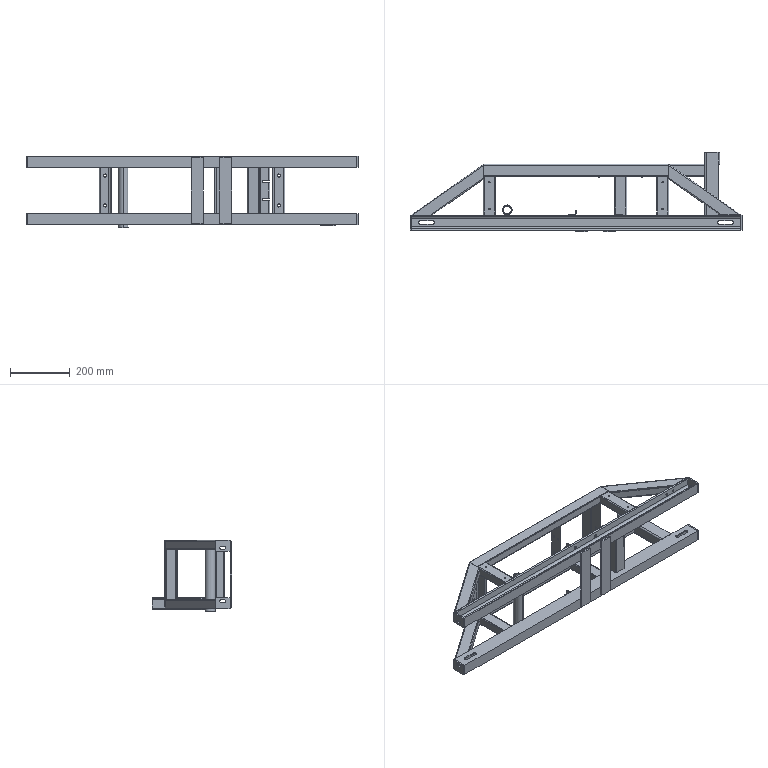Part | SolidWorks | 27 solids | 445 faces | box 1110 x 265 x 240 mm | volume 2438739 mm3 | plane 251 | cylinder 186 | cone 8 | commonest cylinder face diameters 6 x52 1 x40 7 x20 9 x16 10.5 x16 12 x12